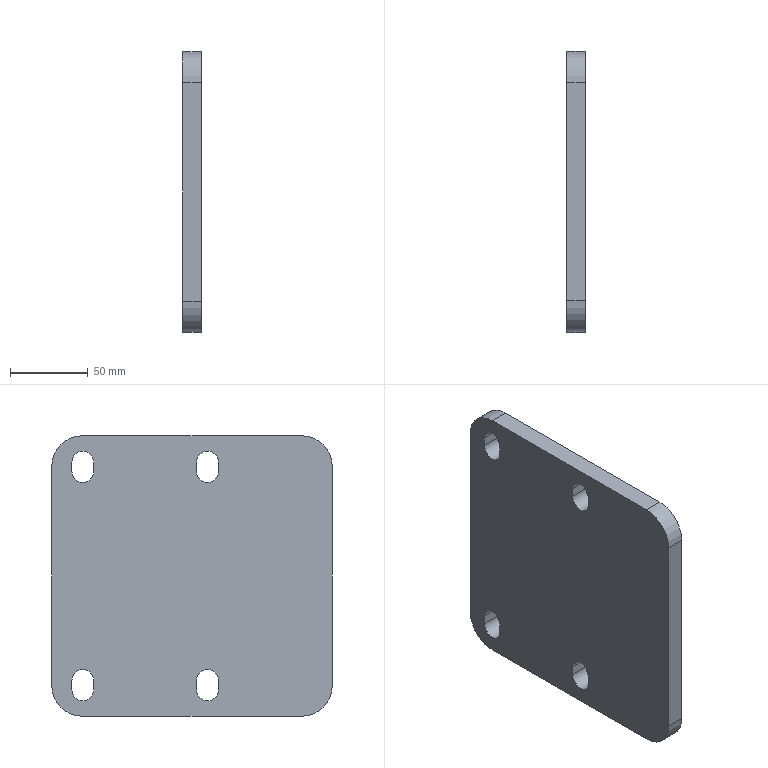Part | STEP file | mounting plate--000.001--20240925 | 1 solid | 26 faces | box 12 x 180 x 180 mm | volume 373259 mm3 | plane 14 | cylinder 12 | commonest cylinder face diameters 14 x8 40 x4